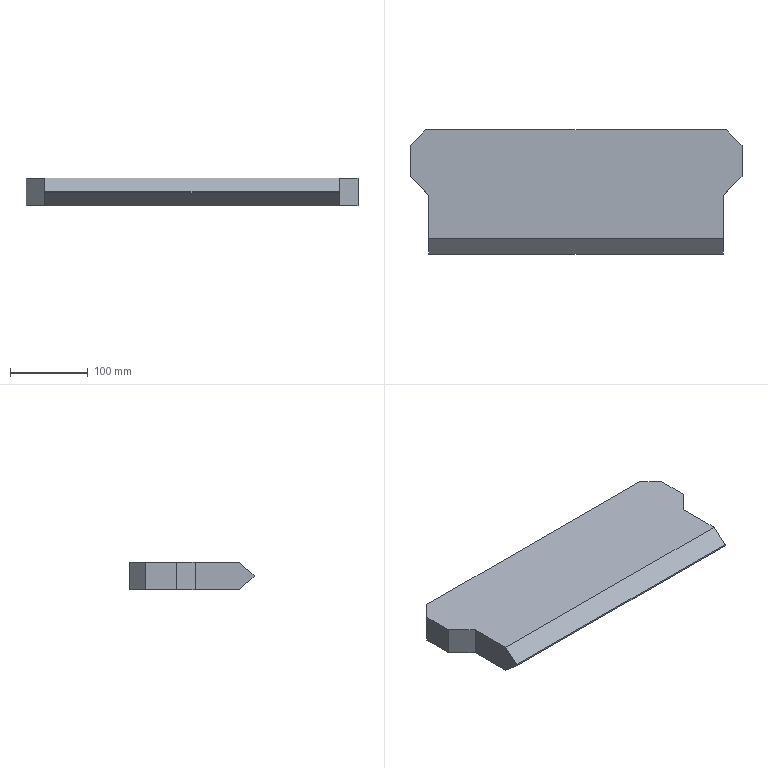Part | SolidWorks | features Extrusion 1, ICE 1 | 1 solid | 14 faces | box 428 x 160 x 36 mm | volume 2167938 mm3 | plane 14
STEP:
#1=CARTESIAN_POINT('',(214.,60.,-18.));
#2=VERTEX_POINT('',#1);
#3=CARTESIAN_POINT('',(194.,80.,-18.));
#4=VERTEX_POINT('',#3);
#5=CARTESIAN_POINT('',(194.,80.,-18.));
#6=DIRECTION('',(-0.7071,0.7071,0.));
#7=VECTOR('',#6,1000.);
#8=LINE('',#5,#7);
#9=EDGE_CURVE('',#2,#4,#8,.T.);
#10=ORIENTED_EDGE('',*,*,#9,.T.);
#11=CARTESIAN_POINT('',(194.,80.,18.));
#12=VERTEX_POINT('',#11);
#13=CARTESIAN_POINT('',(194.,80.,18.));
#14=DIRECTION('',(0.,0.,-1.));
#15=VECTOR('',#14,1000.);
#16=LINE('',#13,#15);
#17=EDGE_CURVE('',#12,#4,#16,.T.);
#18=ORIENTED_EDGE('',*,*,#17,.F.);
#19=CARTESIAN_POINT('',(214.,60.,18.));
#20=VERTEX_POINT('',#19);
#21=CARTESIAN_POINT('',(194.,80.,18.));
#22=DIRECTION('',(-0.7071,0.7071,0.));
#23=VECTOR('',#22,1000.);
#24=LINE('',#21,#23);
#25=EDGE_CURVE('',#20,#12,#24,.T.);
#26=ORIENTED_EDGE('',*,*,#25,.F.);
#27=CARTESIAN_POINT('',(214.,60.,18.));
#28=DIRECTION('',(0.,0.,-1.));
#29=VECTOR('',#28,1000.);
#30=LINE('',#27,#29);
#31=EDGE_CURVE('',#20,#2,#30,.T.);
#32=ORIENTED_EDGE('',*,*,#31,.T.);
#33=EDGE_LOOP('',(#10,#18,#26,#32));
#34=FACE_OUTER_BOUND('',#33,.T.);
#35=CARTESIAN_POINT('',(194.,80.,18.));
#36=DIRECTION('',(-0.7071,-0.7071,0.));
#37=DIRECTION('',(0.7071,-0.7071,0.));
#38=AXIS2_PLACEMENT_3D('',#35,#36,#37);
#39=PLANE('',#38);
#40=ADVANCED_FACE('',(#34),#39,.F.);
#41=CARTESIAN_POINT('',(-194.,80.,-18.));
#42=VERTEX_POINT('',#41);
#43=CARTESIAN_POINT('',(-194.,80.,-18.));
#44=DIRECTION('',(-1.,0.,0.));
#45=VECTOR('',#44,1000.);
#46=LINE('',#43,#45);
#47=EDGE_CURVE('',#4,#42,#46,.T.);
#48=ORIENTED_EDGE('',*,*,#47,.T.);
#49=CARTESIAN_POINT('',(-194.,80.,18.));
#50=VERTEX_POINT('',#49);
#51=CARTESIAN_POINT('',(-194.,80.,18.));
#52=DIRECTION('',(0.,0.,-1.));
#53=VECTOR('',#52,1000.);
#54=LINE('',#51,#53);
#55=EDGE_CURVE('',#50,#42,#54,.T.);
#56=ORIENTED_EDGE('',*,*,#55,.F.);
#57=CARTESIAN_POINT('',(-194.,80.,18.));
#58=DIRECTION('',(-1.,0.,0.));
#59=VECTOR('',#58,1000.);
#60=LINE('',#57,#59);
#61=EDGE_CURVE('',#12,#50,#60,.T.);
#62=ORIENTED_EDGE('',*,*,#61,.F.);
#63=ORIENTED_EDGE('',*,*,#17,.T.);
#64=EDGE_LOOP('',(#48,#56,#62,#63));
#65=FACE_OUTER_BOUND('',#64,.T.);
#66=CARTESIAN_POINT('',(-194.,80.,18.));
#67=DIRECTION('',(0.,-1.,0.));
#68=DIRECTION('',(1.,0.,0.));
#69=AXIS2_PLACEMENT_3D('',#66,#67,#68);
#70=PLANE('',#69);
#71=ADVANCED_FACE('',(#65),#70,.F.);
#72=CARTESIAN_POINT('',(-214.,60.,-18.));
#73=VERTEX_POINT('',#72);
#74=CARTESIAN_POINT('',(-194.,80.,-18.));
#75=DIRECTION('',(-0.7071,-0.7071,0.));
#76=VECTOR('',#75,1000.);
#77=LINE('',#74,#76);
#78=EDGE_CURVE('',#42,#73,#77,.T.);
#79=ORIENTED_EDGE('',*,*,#78,.T.);
#80=CARTESIAN_POINT('',(-214.,60.,18.));
#81=VERTEX_POINT('',#80);
#82=CARTESIAN_POINT('',(-214.,60.,18.));
#83=DIRECTION('',(0.,0.,-1.));
#84=VECTOR('',#83,1000.);
#85=LINE('',#82,#84);
#86=EDGE_CURVE('',#81,#73,#85,.T.);
#87=ORIENTED_EDGE('',*,*,#86,.F.);
#88=CARTESIAN_POINT('',(-194.,80.,18.));
#89=DIRECTION('',(-0.7071,-0.7071,0.));
#90=VECTOR('',#89,1000.);
#91=LINE('',#88,#90);
#92=EDGE_CURVE('',#50,#81,#91,.T.);
#93=ORIENTED_EDGE('',*,*,#92,.F.);
#94=ORIENTED_EDGE('',*,*,#55,.T.);
#95=EDGE_LOOP('',(#79,#87,#93,#94));
#96=FACE_OUTER_BOUND('',#95,.T.);
#97=CARTESIAN_POINT('',(-194.,80.,18.));
#98=DIRECTION('',(0.7071,-0.7071,0.));
#99=DIRECTION('',(0.7071,0.7071,0.));
#100=AXIS2_PLACEMENT_3D('',#97,#98,#99);
#101=PLANE('',#100);
#102=ADVANCED_FACE('',(#96),#101,.F.);
#103=CARTESIAN_POINT('',(-214.,20.,-18.));
#104=VERTEX_POINT('',#103);
#105=CARTESIAN_POINT('',(-214.,60.,-18.));
#106=DIRECTION('',(0.,-1.,0.));
#107=VECTOR('',#106,1000.);
#108=LINE('',#105,#107);
#109=EDGE_CURVE('',#73,#104,#108,.T.);
#110=ORIENTED_EDGE('',*,*,#109,.T.);
#111=CARTESIAN_POINT('',(-214.,20.,18.));
#112=VERTEX_POINT('',#111);
#113=CARTESIAN_POINT('',(-214.,20.,18.));
#114=DIRECTION('',(0.,0.,-1.));
#115=VECTOR('',#114,1000.);
#116=LINE('',#113,#115);
#117=EDGE_CURVE('',#112,#104,#116,.T.);
#118=ORIENTED_EDGE('',*,*,#117,.F.);
#119=CARTESIAN_POINT('',(-214.,60.,18.));
#120=DIRECTION('',(0.,-1.,0.));
#121=VECTOR('',#120,1000.);
#122=LINE('',#119,#121);
#123=EDGE_CURVE('',#81,#112,#122,.T.);
#124=ORIENTED_EDGE('',*,*,#123,.F.);
#125=ORIENTED_EDGE('',*,*,#86,.T.);
#126=EDGE_LOOP('',(#110,#118,#124,#125));
#127=FACE_OUTER_BOUND('',#126,.T.);
#128=CARTESIAN_POINT('',(-214.,60.,18.));
#129=DIRECTION('',(1.,0.,0.));
#130=DIRECTION('',(0.,0.,-1.));
#131=AXIS2_PLACEMENT_3D('',#128,#129,#130);
#132=PLANE('',#131);
#133=ADVANCED_FACE('',(#127),#132,.F.);
#134=CARTESIAN_POINT('',(-190.,-4.,-18.));
#135=VERTEX_POINT('',#134);
#136=CARTESIAN_POINT('',(-214.,20.,-18.));
#137=DIRECTION('',(0.7071,-0.7071,0.));
#138=VECTOR('',#137,1000.);
#139=LINE('',#136,#138);
#140=EDGE_CURVE('',#104,#135,#139,.T.);
#141=ORIENTED_EDGE('',*,*,#140,.T.);
#142=CARTESIAN_POINT('',(-190.,-4.,18.));
#143=VERTEX_POINT('',#142);
#144=CARTESIAN_POINT('',(-190.,-4.,18.));
#145=DIRECTION('',(0.,0.,-1.));
#146=VECTOR('',#145,1000.);
#147=LINE('',#144,#146);
#148=EDGE_CURVE('',#143,#135,#147,.T.);
#149=ORIENTED_EDGE('',*,*,#148,.F.);
#150=CARTESIAN_POINT('',(-214.,20.,18.));
#151=DIRECTION('',(0.7071,-0.7071,0.));
#152=VECTOR('',#151,1000.);
#153=LINE('',#150,#152);
#154=EDGE_CURVE('',#112,#143,#153,.T.);
#155=ORIENTED_EDGE('',*,*,#154,.F.);
#156=ORIENTED_EDGE('',*,*,#117,.T.);
#157=EDGE_LOOP('',(#141,#149,#155,#156));
#158=FACE_OUTER_BOUND('',#157,.T.);
#159=CARTESIAN_POINT('',(-214.,20.,18.));
#160=DIRECTION('',(0.7071,0.7071,0.));
#161=DIRECTION('',(-0.7071,0.7071,0.));
#162=AXIS2_PLACEMENT_3D('',#159,#160,#161);
#163=PLANE('',#162);
#164=ADVANCED_FACE('',(#158),#163,.F.);
#165=CARTESIAN_POINT('',(-190.,-59.74,-18.));
#166=VERTEX_POINT('',#165);
#167=CARTESIAN_POINT('',(-190.,-4.,-18.));
#168=DIRECTION('',(0.,-1.,0.));
#169=VECTOR('',#168,1000.);
#170=LINE('',#167,#169);
#171=EDGE_CURVE('',#135,#166,#170,.T.);
#172=ORIENTED_EDGE('',*,*,#171,.T.);
#173=CARTESIAN_POINT('',(-190.,-80.,-1.));
#174=VERTEX_POINT('',#173);
#175=CARTESIAN_POINT('',(-190.,-44.757,-30.572));
#176=DIRECTION('',(0.,-0.766,0.6428));
#177=VECTOR('',#176,1000.);
#178=LINE('',#175,#177);
#179=EDGE_CURVE('',#166,#174,#178,.T.);
#180=ORIENTED_EDGE('',*,*,#179,.T.);
#181=CARTESIAN_POINT('',(-190.,-80.,1.));
#182=VERTEX_POINT('',#181);
#183=CARTESIAN_POINT('',(-190.,-80.,18.));
#184=DIRECTION('',(0.,0.,-1.));
#185=VECTOR('',#184,1000.);
#186=LINE('',#183,#185);
#187=EDGE_CURVE('',#182,#174,#186,.T.);
#188=ORIENTED_EDGE('',*,*,#187,.F.);
#189=CARTESIAN_POINT('',(-190.,-59.74,18.));
#190=VERTEX_POINT('',#189);
#191=CARTESIAN_POINT('',(-190.,-27.031,45.447));
#192=DIRECTION('',(0.,0.766,0.6428));
#193=VECTOR('',#192,1000.);
#194=LINE('',#191,#193);
#195=EDGE_CURVE('',#182,#190,#194,.T.);
#196=ORIENTED_EDGE('',*,*,#195,.T.);
#197=CARTESIAN_POINT('',(-190.,-4.,18.));
#198=DIRECTION('',(0.,-1.,0.));
#199=VECTOR('',#198,1000.);
#200=LINE('',#197,#199);
#201=EDGE_CURVE('',#143,#190,#200,.T.);
#202=ORIENTED_EDGE('',*,*,#201,.F.);
#203=ORIENTED_EDGE('',*,*,#148,.T.);
#204=EDGE_LOOP('',(#172,#180,#188,#196,#202,#203));
#205=FACE_OUTER_BOUND('',#204,.T.);
#206=CARTESIAN_POINT('',(-190.,-4.,18.));
#207=DIRECTION('',(1.,0.,0.));
#208=DIRECTION('',(0.,0.,-1.));
#209=AXIS2_PLACEMENT_3D('',#206,#207,#208);
#210=PLANE('',#209);
#211=ADVANCED_FACE('',(#205),#210,.F.);
#212=ORIENTED_EDGE('',*,*,#187,.T.);
#213=CARTESIAN_POINT('',(190.,-80.,-1.));
#214=VERTEX_POINT('',#213);
#215=CARTESIAN_POINT('',(-214.,-80.,-1.));
#216=DIRECTION('',(1.,0.,0.));
#217=VECTOR('',#216,1000.);
#218=LINE('',#215,#217);
#219=EDGE_CURVE('',#174,#214,#218,.T.);
#220=ORIENTED_EDGE('',*,*,#219,.T.);
#221=CARTESIAN_POINT('',(190.,-80.,1.));
#222=VERTEX_POINT('',#221);
#223=CARTESIAN_POINT('',(190.,-80.,18.));
#224=DIRECTION('',(0.,0.,-1.));
#225=VECTOR('',#224,1000.);
#226=LINE('',#223,#225);
#227=EDGE_CURVE('',#222,#214,#226,.T.);
#228=ORIENTED_EDGE('',*,*,#227,.F.);
#229=CARTESIAN_POINT('',(-214.,-80.,1.));
#230=DIRECTION('',(1.,0.,0.));
#231=VECTOR('',#230,1000.);
#232=LINE('',#229,#231);
#233=EDGE_CURVE('',#182,#222,#232,.T.);
#234=ORIENTED_EDGE('',*,*,#233,.F.);
#235=EDGE_LOOP('',(#212,#220,#228,#234));
#236=FACE_OUTER_BOUND('',#235,.T.);
#237=CARTESIAN_POINT('',(190.,-80.,18.));
#238=DIRECTION('',(0.,1.,0.));
#239=DIRECTION('',(0.,0.,1.));
#240=AXIS2_PLACEMENT_3D('',#237,#238,#239);
#241=PLANE('',#240);
#242=ADVANCED_FACE('',(#236),#241,.F.);
#243=ORIENTED_EDGE('',*,*,#227,.T.);
#244=CARTESIAN_POINT('',(190.,-59.74,-18.));
#245=VERTEX_POINT('',#244);
#246=CARTESIAN_POINT('',(190.,-44.757,-30.572));
#247=DIRECTION('',(0.,0.766,-0.6428));
#248=VECTOR('',#247,1000.);
#249=LINE('',#246,#248);
#250=EDGE_CURVE('',#214,#245,#249,.T.);
#251=ORIENTED_EDGE('',*,*,#250,.T.);
#252=CARTESIAN_POINT('',(190.,-4.,-18.));
#253=VERTEX_POINT('',#252);
#254=CARTESIAN_POINT('',(190.,-4.,-18.));
#255=DIRECTION('',(0.,1.,0.));
#256=VECTOR('',#255,1000.);
#257=LINE('',#254,#256);
#258=EDGE_CURVE('',#245,#253,#257,.T.);
#259=ORIENTED_EDGE('',*,*,#258,.T.);
#260=CARTESIAN_POINT('',(190.,-4.,18.));
#261=VERTEX_POINT('',#260);
#262=CARTESIAN_POINT('',(190.,-4.,18.));
#263=DIRECTION('',(0.,0.,-1.));
#264=VECTOR('',#263,1000.);
#265=LINE('',#262,#264);
#266=EDGE_CURVE('',#261,#253,#265,.T.);
#267=ORIENTED_EDGE('',*,*,#266,.F.);
#268=CARTESIAN_POINT('',(190.,-59.74,18.));
#269=VERTEX_POINT('',#268);
#270=CARTESIAN_POINT('',(190.,-4.,18.));
#271=DIRECTION('',(0.,1.,0.));
#272=VECTOR('',#271,1000.);
#273=LINE('',#270,#272);
#274=EDGE_CURVE('',#269,#261,#273,.T.);
#275=ORIENTED_EDGE('',*,*,#274,.F.);
#276=CARTESIAN_POINT('',(190.,-27.031,45.447));
#277=DIRECTION('',(0.,-0.766,-0.6428));
#278=VECTOR('',#277,1000.);
#279=LINE('',#276,#278);
#280=EDGE_CURVE('',#269,#222,#279,.T.);
#281=ORIENTED_EDGE('',*,*,#280,.T.);
#282=EDGE_LOOP('',(#243,#251,#259,#267,#275,#281));
#283=FACE_OUTER_BOUND('',#282,.T.);
#284=CARTESIAN_POINT('',(190.,-4.,18.));
#285=DIRECTION('',(-1.,0.,0.));
#286=DIRECTION('',(0.,0.,1.));
#287=AXIS2_PLACEMENT_3D('',#284,#285,#286);
#288=PLANE('',#287);
#289=ADVANCED_FACE('',(#283),#288,.F.);
#290=CARTESIAN_POINT('',(214.,20.,-18.));
#291=VERTEX_POINT('',#290);
#292=CARTESIAN_POINT('',(214.,20.,-18.));
#293=DIRECTION('',(0.7071,0.7071,0.));
#294=VECTOR('',#293,1000.);
#295=LINE('',#292,#294);
#296=EDGE_CURVE('',#253,#291,#295,.T.);
#297=ORIENTED_EDGE('',*,*,#296,.T.);
#298=CARTESIAN_POINT('',(214.,20.,18.));
#299=VERTEX_POINT('',#298);
#300=CARTESIAN_POINT('',(214.,20.,18.));
#301=DIRECTION('',(0.,0.,-1.));
#302=VECTOR('',#301,1000.);
#303=LINE('',#300,#302);
#304=EDGE_CURVE('',#299,#291,#303,.T.);
#305=ORIENTED_EDGE('',*,*,#304,.F.);
#306=CARTESIAN_POINT('',(214.,20.,18.));
#307=DIRECTION('',(0.7071,0.7071,0.));
#308=VECTOR('',#307,1000.);
#309=LINE('',#306,#308);
#310=EDGE_CURVE('',#261,#299,#309,.T.);
#311=ORIENTED_EDGE('',*,*,#310,.F.);
#312=ORIENTED_EDGE('',*,*,#266,.T.);
#313=EDGE_LOOP('',(#297,#305,#311,#312));
#314=FACE_OUTER_BOUND('',#313,.T.);
#315=CARTESIAN_POINT('',(214.,20.,18.));
#316=DIRECTION('',(-0.7071,0.7071,0.));
#317=DIRECTION('',(-0.7071,-0.7071,0.));
#318=AXIS2_PLACEMENT_3D('',#315,#316,#317);
#319=PLANE('',#318);
#320=ADVANCED_FACE('',(#314),#319,.F.);
#321=CARTESIAN_POINT('',(214.,60.,-18.));
#322=DIRECTION('',(0.,1.,0.));
#323=VECTOR('',#322,1000.);
#324=LINE('',#321,#323);
#325=EDGE_CURVE('',#291,#2,#324,.T.);
#326=ORIENTED_EDGE('',*,*,#325,.T.);
#327=ORIENTED_EDGE('',*,*,#31,.F.);
#328=CARTESIAN_POINT('',(214.,60.,18.));
#329=DIRECTION('',(0.,1.,0.));
#330=VECTOR('',#329,1000.);
#331=LINE('',#328,#330);
#332=EDGE_CURVE('',#299,#20,#331,.T.);
#333=ORIENTED_EDGE('',*,*,#332,.F.);
#334=ORIENTED_EDGE('',*,*,#304,.T.);
#335=EDGE_LOOP('',(#326,#327,#333,#334));
#336=FACE_OUTER_BOUND('',#335,.T.);
#337=CARTESIAN_POINT('',(214.,60.,18.));
#338=DIRECTION('',(-1.,0.,0.));
#339=DIRECTION('',(0.,0.,1.));
#340=AXIS2_PLACEMENT_3D('',#337,#338,#339);
#341=PLANE('',#340);
#342=ADVANCED_FACE('',(#336),#341,.F.);
#343=ORIENTED_EDGE('',*,*,#201,.T.);
#344=CARTESIAN_POINT('',(234.,-59.74,18.));
#345=DIRECTION('',(1.,0.,0.));
#346=VECTOR('',#345,1000.);
#347=LINE('',#344,#346);
#348=EDGE_CURVE('',#190,#269,#347,.T.);
#349=ORIENTED_EDGE('',*,*,#348,.T.);
#350=ORIENTED_EDGE('',*,*,#274,.T.);
#351=ORIENTED_EDGE('',*,*,#310,.T.);
#352=ORIENTED_EDGE('',*,*,#332,.T.);
#353=ORIENTED_EDGE('',*,*,#25,.T.);
#354=ORIENTED_EDGE('',*,*,#61,.T.);
#355=ORIENTED_EDGE('',*,*,#92,.T.);
#356=ORIENTED_EDGE('',*,*,#123,.T.);
#357=ORIENTED_EDGE('',*,*,#154,.T.);
#358=EDGE_LOOP('',(#343,#349,#350,#351,#352,#353,#354,#355,#356,#357));
#359=FACE_OUTER_BOUND('',#358,.T.);
#360=CARTESIAN_POINT('',(234.,40.,18.));
#361=DIRECTION('',(0.,0.,-1.));
#362=DIRECTION('',(-1.,0.,0.));
#363=AXIS2_PLACEMENT_3D('',#360,#361,#362);
#364=PLANE('',#363);
#365=ADVANCED_FACE('',(#359),#364,.F.);
#366=CARTESIAN_POINT('',(234.,-59.74,-18.));
#367=DIRECTION('',(1.,0.,0.));
#368=VECTOR('',#367,1000.);
#369=LINE('',#366,#368);
#370=EDGE_CURVE('',#166,#245,#369,.T.);
#371=ORIENTED_EDGE('',*,*,#370,.F.);
#372=ORIENTED_EDGE('',*,*,#171,.F.);
#373=ORIENTED_EDGE('',*,*,#140,.F.);
#374=ORIENTED_EDGE('',*,*,#109,.F.);
#375=ORIENTED_EDGE('',*,*,#78,.F.);
#376=ORIENTED_EDGE('',*,*,#47,.F.);
#377=ORIENTED_EDGE('',*,*,#9,.F.);
#378=ORIENTED_EDGE('',*,*,#325,.F.);
#379=ORIENTED_EDGE('',*,*,#296,.F.);
#380=ORIENTED_EDGE('',*,*,#258,.F.);
#381=EDGE_LOOP('',(#371,#372,#373,#374,#375,#376,#377,#378,#379,#380));
#382=FACE_OUTER_BOUND('',#381,.T.);
#383=CARTESIAN_POINT('',(234.,40.,-18.));
#384=DIRECTION('',(0.,0.,-1.));
#385=DIRECTION('',(-1.,0.,0.));
#386=AXIS2_PLACEMENT_3D('',#383,#384,#385);
#387=PLANE('',#386);
#388=ADVANCED_FACE('',(#382),#387,.T.);
#389=ORIENTED_EDGE('',*,*,#233,.T.);
#390=ORIENTED_EDGE('',*,*,#280,.F.);
#391=ORIENTED_EDGE('',*,*,#348,.F.);
#392=ORIENTED_EDGE('',*,*,#195,.F.);
#393=EDGE_LOOP('',(#389,#390,#391,#392));
#394=FACE_OUTER_BOUND('',#393,.T.);
#395=CARTESIAN_POINT('',(-214.,-80.,1.));
#396=DIRECTION('',(0.,0.6428,-0.766));
#397=DIRECTION('',(0.,0.766,0.6428));
#398=AXIS2_PLACEMENT_3D('',#395,#396,#397);
#399=PLANE('',#398);
#400=ADVANCED_FACE('',(#394),#399,.F.);
#401=ORIENTED_EDGE('',*,*,#370,.T.);
#402=ORIENTED_EDGE('',*,*,#250,.F.);
#403=ORIENTED_EDGE('',*,*,#219,.F.);
#404=ORIENTED_EDGE('',*,*,#179,.F.);
#405=EDGE_LOOP('',(#401,#402,#403,#404));
#406=FACE_OUTER_BOUND('',#405,.T.);
#407=CARTESIAN_POINT('',(-214.,-80.,-1.));
#408=DIRECTION('',(0.,0.6428,0.766));
#409=DIRECTION('',(0.,-0.766,0.6428));
#410=AXIS2_PLACEMENT_3D('',#407,#408,#409);
#411=PLANE('',#410);
#412=ADVANCED_FACE('',(#406),#411,.F.);
#413=CLOSED_SHELL('',(#40,#71,#102,#133,#164,#211,#242,#289,#320,#342,#365,#388,#400,#412));
#414=MANIFOLD_SOLID_BREP('',#413);
#415=CARTESIAN_POINT('',(0.,0.,0.));
#416=DIRECTION('',(0.,0.,1.));
#417=DIRECTION('',(1.,0.,0.));
#418=AXIS2_PLACEMENT_3D('',#415,#416,#417);
#419=(LENGTH_UNIT()NAMED_UNIT(*)SI_UNIT(.MILLI.,.METRE.));
#420=UNCERTAINTY_MEASURE_WITH_UNIT(LENGTH_MEASURE(0.00001),#419,'','');
#421=(NAMED_UNIT(*)PLANE_ANGLE_UNIT()SI_UNIT($,.RADIAN.));
#422=(NAMED_UNIT(*)SI_UNIT($,.STERADIAN.)SOLID_ANGLE_UNIT());
#423=(GEOMETRIC_REPRESENTATION_CONTEXT(3)GLOBAL_UNCERTAINTY_ASSIGNED_CONTEXT((#420))GLOBAL_UNIT_ASSIGNED_CONTEXT((#419,#421,#422))REPRESENTATION_CONTEXT('',''));
#424=ADVANCED_BREP_SHAPE_REPRESENTATION('',(#414,#418),#423);